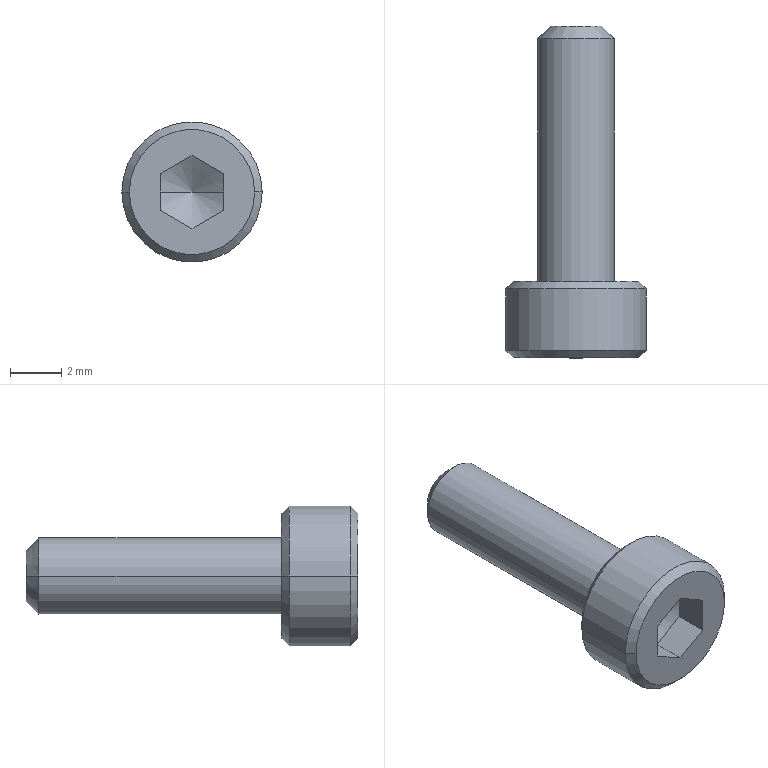Part | STEP file | BB62-M3-10L-17 | 1 solid | 27 faces | box 5.5 x 13 x 5.5 mm | volume 130.673 mm3 | plane 15 | cone 8 | cylinder 4 | commonest cylinder face diameters 3 x2 5.5 x2
STEP:
#1=CARTESIAN_POINT('',(0.,-0.8715,0.));
#2=VERTEX_POINT('',#1);
#3=CARTESIAN_POINT('',(1.435,-1.7,0.));
#4=VERTEX_POINT('',#3);
#5=CARTESIAN_POINT('',(0.,-0.8715,0.));
#6=DIRECTION('',(0.866,-0.5,0.));
#7=VECTOR('',#6,1000.);
#8=LINE('',#5,#7);
#9=EDGE_CURVE('',#2,#4,#8,.T.);
#10=ORIENTED_EDGE('',*,*,#9,.F.);
#11=CARTESIAN_POINT('',(-1.435,-1.7,0.));
#12=VERTEX_POINT('',#11);
#13=CARTESIAN_POINT('',(0.,-0.8715,0.));
#14=DIRECTION('',(-0.866,-0.5,0.));
#15=VECTOR('',#14,1000.);
#16=LINE('',#13,#15);
#17=EDGE_CURVE('',#2,#12,#16,.T.);
#18=ORIENTED_EDGE('',*,*,#17,.T.);
#19=CARTESIAN_POINT('',(-1.243,-1.7,-0.7175));
#20=VERTEX_POINT('',#19);
#21=CARTESIAN_POINT('',(0.,-1.7,0.));
#22=DIRECTION('',(0.,-1.,0.));
#23=DIRECTION('',(-1.,0.,0.));
#24=AXIS2_PLACEMENT_3D('',#21,#22,#23);
#25=CIRCLE('',#24,1.435);
#26=EDGE_CURVE('',#12,#20,#25,.T.);
#27=ORIENTED_EDGE('',*,*,#26,.T.);
#28=CARTESIAN_POINT('',(0.,-1.7,-1.435));
#29=VERTEX_POINT('',#28);
#30=CARTESIAN_POINT('',(0.,-1.7,0.));
#31=DIRECTION('',(0.,-1.,0.));
#32=DIRECTION('',(-1.,0.,0.));
#33=AXIS2_PLACEMENT_3D('',#30,#31,#32);
#34=CIRCLE('',#33,1.435);
#35=EDGE_CURVE('',#20,#29,#34,.T.);
#36=ORIENTED_EDGE('',*,*,#35,.T.);
#37=CARTESIAN_POINT('',(1.243,-1.7,-0.7175));
#38=VERTEX_POINT('',#37);
#39=CARTESIAN_POINT('',(0.,-1.7,0.));
#40=DIRECTION('',(0.,-1.,0.));
#41=DIRECTION('',(-1.,0.,0.));
#42=AXIS2_PLACEMENT_3D('',#39,#40,#41);
#43=CIRCLE('',#42,1.435);
#44=EDGE_CURVE('',#29,#38,#43,.T.);
#45=ORIENTED_EDGE('',*,*,#44,.T.);
#46=CARTESIAN_POINT('',(0.,-1.7,0.));
#47=DIRECTION('',(0.,-1.,0.));
#48=DIRECTION('',(-1.,0.,0.));
#49=AXIS2_PLACEMENT_3D('',#46,#47,#48);
#50=CIRCLE('',#49,1.435);
#51=EDGE_CURVE('',#38,#4,#50,.T.);
#52=ORIENTED_EDGE('',*,*,#51,.T.);
#53=EDGE_LOOP('',(#10,#18,#27,#36,#45,#52));
#54=FACE_OUTER_BOUND('',#53,.T.);
#55=CARTESIAN_POINT('',(0.,-1000.872,0.));
#56=DIRECTION('',(0.,-1.,0.));
#57=DIRECTION('',(1.,0.,0.));
#58=AXIS2_PLACEMENT_3D('',#55,#56,#57);
#59=CONICAL_SURFACE('',#58,1732.051,1.047);
#60=ADVANCED_FACE('',(#54),#59,.F.);
#61=CARTESIAN_POINT('',(-1.,10.,0.));
#62=VERTEX_POINT('',#61);
#63=CARTESIAN_POINT('',(1.,10.,0.));
#64=VERTEX_POINT('',#63);
#65=CARTESIAN_POINT('',(0.,10.,0.));
#66=DIRECTION('',(0.,1.,0.));
#67=DIRECTION('',(1.,0.,0.));
#68=AXIS2_PLACEMENT_3D('',#65,#66,#67);
#69=CIRCLE('',#68,1.);
#70=EDGE_CURVE('',#62,#64,#69,.T.);
#71=ORIENTED_EDGE('',*,*,#70,.F.);
#72=CARTESIAN_POINT('',(-1.5,9.5,0.));
#73=VERTEX_POINT('',#72);
#74=CARTESIAN_POINT('',(-1.,10.,0.));
#75=DIRECTION('',(-0.7071,-0.7071,0.));
#76=VECTOR('',#75,1000.);
#77=LINE('',#74,#76);
#78=EDGE_CURVE('',#62,#73,#77,.T.);
#79=ORIENTED_EDGE('',*,*,#78,.T.);
#80=CARTESIAN_POINT('',(1.5,9.5,0.));
#81=VERTEX_POINT('',#80);
#82=CARTESIAN_POINT('',(0.,9.5,0.));
#83=DIRECTION('',(0.,-1.,0.));
#84=DIRECTION('',(-1.,0.,0.));
#85=AXIS2_PLACEMENT_3D('',#82,#83,#84);
#86=CIRCLE('',#85,1.5);
#87=EDGE_CURVE('',#81,#73,#86,.T.);
#88=ORIENTED_EDGE('',*,*,#87,.F.);
#89=CARTESIAN_POINT('',(1.,10.,0.));
#90=DIRECTION('',(0.7071,-0.7071,0.));
#91=VECTOR('',#90,1000.);
#92=LINE('',#89,#91);
#93=EDGE_CURVE('',#64,#81,#92,.T.);
#94=ORIENTED_EDGE('',*,*,#93,.F.);
#95=EDGE_LOOP('',(#71,#79,#88,#94));
#96=FACE_OUTER_BOUND('',#95,.T.);
#97=CARTESIAN_POINT('',(0.,10.,0.));
#98=DIRECTION('',(0.,-1.,0.));
#99=DIRECTION('',(1.,0.,0.));
#100=AXIS2_PLACEMENT_3D('',#97,#98,#99);
#101=CONICAL_SURFACE('',#100,1.,0.7854);
#102=ADVANCED_FACE('',(#96),#101,.T.);
#103=ORIENTED_EDGE('',*,*,#87,.T.);
#104=CARTESIAN_POINT('',(-1.5,0.,0.));
#105=VERTEX_POINT('',#104);
#106=CARTESIAN_POINT('',(-1.5,9.5,0.));
#107=DIRECTION('',(0.,-1.,0.));
#108=VECTOR('',#107,1000.);
#109=LINE('',#106,#108);
#110=EDGE_CURVE('',#73,#105,#109,.T.);
#111=ORIENTED_EDGE('',*,*,#110,.T.);
#112=CARTESIAN_POINT('',(1.5,0.,0.));
#113=VERTEX_POINT('',#112);
#114=CARTESIAN_POINT('',(0.,0.,0.));
#115=DIRECTION('',(0.,-1.,0.));
#116=DIRECTION('',(-1.,0.,0.));
#117=AXIS2_PLACEMENT_3D('',#114,#115,#116);
#118=CIRCLE('',#117,1.5);
#119=EDGE_CURVE('',#113,#105,#118,.T.);
#120=ORIENTED_EDGE('',*,*,#119,.F.);
#121=CARTESIAN_POINT('',(1.5,9.5,0.));
#122=DIRECTION('',(0.,-1.,0.));
#123=VECTOR('',#122,1000.);
#124=LINE('',#121,#123);
#125=EDGE_CURVE('',#81,#113,#124,.T.);
#126=ORIENTED_EDGE('',*,*,#125,.F.);
#127=EDGE_LOOP('',(#103,#111,#120,#126));
#128=FACE_OUTER_BOUND('',#127,.T.);
#129=CARTESIAN_POINT('',(0.,9.5,0.));
#130=DIRECTION('',(0.,-1.,0.));
#131=DIRECTION('',(1.,0.,0.));
#132=AXIS2_PLACEMENT_3D('',#129,#130,#131);
#133=CYLINDRICAL_SURFACE('',#132,1.5);
#134=ADVANCED_FACE('',(#128),#133,.T.);
#135=CARTESIAN_POINT('',(2.45,-3.,0.));
#136=VERTEX_POINT('',#135);
#137=CARTESIAN_POINT('',(-2.45,-3.,0.));
#138=VERTEX_POINT('',#137);
#139=CARTESIAN_POINT('',(0.,-3.,0.));
#140=DIRECTION('',(0.,-1.,0.));
#141=DIRECTION('',(-1.,0.,0.));
#142=AXIS2_PLACEMENT_3D('',#139,#140,#141);
#143=CIRCLE('',#142,2.45);
#144=EDGE_CURVE('',#136,#138,#143,.T.);
#145=ORIENTED_EDGE('',*,*,#144,.F.);
#146=CARTESIAN_POINT('',(2.75,-2.7,0.));
#147=VERTEX_POINT('',#146);
#148=CARTESIAN_POINT('',(2.75,-2.7,0.));
#149=DIRECTION('',(0.7071,0.7071,0.));
#150=VECTOR('',#149,1000.);
#151=LINE('',#148,#150);
#152=EDGE_CURVE('',#136,#147,#151,.T.);
#153=ORIENTED_EDGE('',*,*,#152,.T.);
#154=CARTESIAN_POINT('',(-2.75,-2.7,0.));
#155=VERTEX_POINT('',#154);
#156=CARTESIAN_POINT('',(0.,-2.7,0.));
#157=DIRECTION('',(0.,-1.,0.));
#158=DIRECTION('',(-1.,0.,0.));
#159=AXIS2_PLACEMENT_3D('',#156,#157,#158);
#160=CIRCLE('',#159,2.75);
#161=EDGE_CURVE('',#147,#155,#160,.T.);
#162=ORIENTED_EDGE('',*,*,#161,.T.);
#163=CARTESIAN_POINT('',(-2.75,-2.7,0.));
#164=DIRECTION('',(-0.7071,0.7071,0.));
#165=VECTOR('',#164,1000.);
#166=LINE('',#163,#165);
#167=EDGE_CURVE('',#138,#155,#166,.T.);
#168=ORIENTED_EDGE('',*,*,#167,.F.);
#169=EDGE_LOOP('',(#145,#153,#162,#168));
#170=FACE_OUTER_BOUND('',#169,.T.);
#171=CARTESIAN_POINT('',(0.,-2.7,0.));
#172=DIRECTION('',(0.,1.,0.));
#173=DIRECTION('',(-1.,0.,0.));
#174=AXIS2_PLACEMENT_3D('',#171,#172,#173);
#175=CONICAL_SURFACE('',#174,2.75,0.7854);
#176=ADVANCED_FACE('',(#170),#175,.T.);
#177=ORIENTED_EDGE('',*,*,#161,.F.);
#178=CARTESIAN_POINT('',(2.75,-0.3,0.));
#179=VERTEX_POINT('',#178);
#180=CARTESIAN_POINT('',(2.75,-1.62,0.));
#181=DIRECTION('',(0.,1.,0.));
#182=VECTOR('',#181,1000.);
#183=LINE('',#180,#182);
#184=EDGE_CURVE('',#147,#179,#183,.T.);
#185=ORIENTED_EDGE('',*,*,#184,.T.);
#186=CARTESIAN_POINT('',(-2.75,-0.3,0.));
#187=VERTEX_POINT('',#186);
#188=CARTESIAN_POINT('',(0.,-0.3,0.));
#189=DIRECTION('',(0.,-1.,0.));
#190=DIRECTION('',(-1.,0.,0.));
#191=AXIS2_PLACEMENT_3D('',#188,#189,#190);
#192=CIRCLE('',#191,2.75);
#193=EDGE_CURVE('',#179,#187,#192,.T.);
#194=ORIENTED_EDGE('',*,*,#193,.T.);
#195=CARTESIAN_POINT('',(-2.75,-1.62,0.));
#196=DIRECTION('',(0.,1.,0.));
#197=VECTOR('',#196,1000.);
#198=LINE('',#195,#197);
#199=EDGE_CURVE('',#155,#187,#198,.T.);
#200=ORIENTED_EDGE('',*,*,#199,.F.);
#201=EDGE_LOOP('',(#177,#185,#194,#200));
#202=FACE_OUTER_BOUND('',#201,.T.);
#203=CARTESIAN_POINT('',(0.,-1.62,0.));
#204=DIRECTION('',(0.,1.,0.));
#205=DIRECTION('',(-1.,0.,0.));
#206=AXIS2_PLACEMENT_3D('',#203,#204,#205);
#207=CYLINDRICAL_SURFACE('',#206,2.75);
#208=ADVANCED_FACE('',(#202),#207,.T.);
#209=CARTESIAN_POINT('',(2.45,0.,0.));
#210=VERTEX_POINT('',#209);
#211=CARTESIAN_POINT('',(-2.45,0.,0.));
#212=VERTEX_POINT('',#211);
#213=CARTESIAN_POINT('',(0.,0.,0.));
#214=DIRECTION('',(0.,-1.,0.));
#215=DIRECTION('',(-1.,0.,0.));
#216=AXIS2_PLACEMENT_3D('',#213,#214,#215);
#217=CIRCLE('',#216,2.45);
#218=EDGE_CURVE('',#210,#212,#217,.T.);
#219=ORIENTED_EDGE('',*,*,#218,.T.);
#220=CARTESIAN_POINT('',(-2.45,0.,0.));
#221=DIRECTION('',(-0.7071,-0.7071,0.));
#222=VECTOR('',#221,1000.);
#223=LINE('',#220,#222);
#224=EDGE_CURVE('',#212,#187,#223,.T.);
#225=ORIENTED_EDGE('',*,*,#224,.T.);
#226=ORIENTED_EDGE('',*,*,#193,.F.);
#227=CARTESIAN_POINT('',(2.45,0.,0.));
#228=DIRECTION('',(0.7071,-0.7071,0.));
#229=VECTOR('',#228,1000.);
#230=LINE('',#227,#229);
#231=EDGE_CURVE('',#210,#179,#230,.T.);
#232=ORIENTED_EDGE('',*,*,#231,.F.);
#233=EDGE_LOOP('',(#219,#225,#226,#232));
#234=FACE_OUTER_BOUND('',#233,.T.);
#235=CARTESIAN_POINT('',(0.,0.,0.));
#236=DIRECTION('',(0.,-1.,0.));
#237=DIRECTION('',(1.,0.,0.));
#238=AXIS2_PLACEMENT_3D('',#235,#236,#237);
#239=CONICAL_SURFACE('',#238,2.45,0.7854);
#240=ADVANCED_FACE('',(#234),#239,.T.);
#241=CARTESIAN_POINT('',(0.,-3.,0.));
#242=DIRECTION('',(0.,-1.,0.));
#243=DIRECTION('',(-1.,0.,0.));
#244=AXIS2_PLACEMENT_3D('',#241,#242,#243);
#245=CIRCLE('',#244,2.45);
#246=EDGE_CURVE('',#138,#136,#245,.T.);
#247=ORIENTED_EDGE('',*,*,#246,.T.);
#248=ORIENTED_EDGE('',*,*,#144,.T.);
#249=EDGE_LOOP('',(#247,#248));
#250=FACE_OUTER_BOUND('',#249,.T.);
#251=CARTESIAN_POINT('',(0.,-3.,-1.435));
#252=VERTEX_POINT('',#251);
#253=CARTESIAN_POINT('',(-1.243,-3.,-0.7175));
#254=VERTEX_POINT('',#253);
#255=CARTESIAN_POINT('',(0.,-3.,-1.435));
#256=DIRECTION('',(-0.866,0.,0.5));
#257=VECTOR('',#256,1000.);
#258=LINE('',#255,#257);
#259=EDGE_CURVE('',#252,#254,#258,.T.);
#260=ORIENTED_EDGE('',*,*,#259,.T.);
#261=CARTESIAN_POINT('',(-1.243,-3.,0.7175));
#262=VERTEX_POINT('',#261);
#263=CARTESIAN_POINT('',(-1.243,-3.,-0.7175));
#264=DIRECTION('',(0.,0.,1.));
#265=VECTOR('',#264,1000.);
#266=LINE('',#263,#265);
#267=EDGE_CURVE('',#254,#262,#266,.T.);
#268=ORIENTED_EDGE('',*,*,#267,.T.);
#269=CARTESIAN_POINT('',(0.,-3.,1.435));
#270=VERTEX_POINT('',#269);
#271=CARTESIAN_POINT('',(-1.243,-3.,0.7175));
#272=DIRECTION('',(0.866,0.,0.5));
#273=VECTOR('',#272,1000.);
#274=LINE('',#271,#273);
#275=EDGE_CURVE('',#262,#270,#274,.T.);
#276=ORIENTED_EDGE('',*,*,#275,.T.);
#277=CARTESIAN_POINT('',(1.243,-3.,0.7175));
#278=VERTEX_POINT('',#277);
#279=CARTESIAN_POINT('',(0.,-3.,1.435));
#280=DIRECTION('',(0.866,0.,-0.5));
#281=VECTOR('',#280,1000.);
#282=LINE('',#279,#281);
#283=EDGE_CURVE('',#270,#278,#282,.T.);
#284=ORIENTED_EDGE('',*,*,#283,.T.);
#285=CARTESIAN_POINT('',(1.243,-3.,-0.7175));
#286=VERTEX_POINT('',#285);
#287=CARTESIAN_POINT('',(1.243,-3.,0.7175));
#288=DIRECTION('',(0.,0.,-1.));
#289=VECTOR('',#288,1000.);
#290=LINE('',#287,#289);
#291=EDGE_CURVE('',#278,#286,#290,.T.);
#292=ORIENTED_EDGE('',*,*,#291,.T.);
#293=CARTESIAN_POINT('',(1.243,-3.,-0.7175));
#294=DIRECTION('',(-0.866,0.,-0.5));
#295=VECTOR('',#294,1000.);
#296=LINE('',#293,#295);
#297=EDGE_CURVE('',#286,#252,#296,.T.);
#298=ORIENTED_EDGE('',*,*,#297,.T.);
#299=EDGE_LOOP('',(#260,#268,#276,#284,#292,#298));
#300=FACE_BOUND('',#299,.T.);
#301=CARTESIAN_POINT('',(2.45,-3.,0.));
#302=DIRECTION('',(0.,-1.,0.));
#303=DIRECTION('',(1.,0.,0.));
#304=AXIS2_PLACEMENT_3D('',#301,#302,#303);
#305=PLANE('',#304);
#306=ADVANCED_FACE('',(#250,#300),#305,.T.);
#307=ORIENTED_EDGE('',*,*,#119,.T.);
#308=CARTESIAN_POINT('',(0.,0.,0.));
#309=DIRECTION('',(0.,-1.,0.));
#310=DIRECTION('',(-1.,0.,0.));
#311=AXIS2_PLACEMENT_3D('',#308,#309,#310);
#312=CIRCLE('',#311,1.5);
#313=EDGE_CURVE('',#105,#113,#312,.T.);
#314=ORIENTED_EDGE('',*,*,#313,.T.);
#315=EDGE_LOOP('',(#307,#314));
#316=FACE_BOUND('',#315,.T.);
#317=ORIENTED_EDGE('',*,*,#218,.F.);
#318=CARTESIAN_POINT('',(0.,0.,0.));
#319=DIRECTION('',(0.,-1.,0.));
#320=DIRECTION('',(-1.,0.,0.));
#321=AXIS2_PLACEMENT_3D('',#318,#319,#320);
#322=CIRCLE('',#321,2.45);
#323=EDGE_CURVE('',#212,#210,#322,.T.);
#324=ORIENTED_EDGE('',*,*,#323,.F.);
#325=EDGE_LOOP('',(#317,#324));
#326=FACE_OUTER_BOUND('',#325,.T.);
#327=CARTESIAN_POINT('',(0.,0.,0.));
#328=DIRECTION('',(0.,1.,0.));
#329=DIRECTION('',(-1.,0.,0.));
#330=AXIS2_PLACEMENT_3D('',#327,#328,#329);
#331=PLANE('',#330);
#332=ADVANCED_FACE('',(#316,#326),#331,.T.);
#333=ORIENTED_EDGE('',*,*,#224,.F.);
#334=ORIENTED_EDGE('',*,*,#323,.T.);
#335=ORIENTED_EDGE('',*,*,#231,.T.);
#336=CARTESIAN_POINT('',(0.,-0.3,0.));
#337=DIRECTION('',(0.,-1.,0.));
#338=DIRECTION('',(-1.,0.,0.));
#339=AXIS2_PLACEMENT_3D('',#336,#337,#338);
#340=CIRCLE('',#339,2.75);
#341=EDGE_CURVE('',#187,#179,#340,.T.);
#342=ORIENTED_EDGE('',*,*,#341,.F.);
#343=EDGE_LOOP('',(#333,#334,#335,#342));
#344=FACE_OUTER_BOUND('',#343,.T.);
#345=CARTESIAN_POINT('',(0.,0.,0.));
#346=DIRECTION('',(0.,-1.,0.));
#347=DIRECTION('',(1.,0.,0.));
#348=AXIS2_PLACEMENT_3D('',#345,#346,#347);
#349=CONICAL_SURFACE('',#348,2.45,0.7854);
#350=ADVANCED_FACE('',(#344),#349,.T.);
#351=ORIENTED_EDGE('',*,*,#184,.F.);
#352=CARTESIAN_POINT('',(0.,-2.7,0.));
#353=DIRECTION('',(0.,-1.,0.));
#354=DIRECTION('',(-1.,0.,0.));
#355=AXIS2_PLACEMENT_3D('',#352,#353,#354);
#356=CIRCLE('',#355,2.75);
#357=EDGE_CURVE('',#155,#147,#356,.T.);
#358=ORIENTED_EDGE('',*,*,#357,.F.);
#359=ORIENTED_EDGE('',*,*,#199,.T.);
#360=ORIENTED_EDGE('',*,*,#341,.T.);
#361=EDGE_LOOP('',(#351,#358,#359,#360));
#362=FACE_OUTER_BOUND('',#361,.T.);
#363=CARTESIAN_POINT('',(0.,-1.62,0.));
#364=DIRECTION('',(0.,1.,0.));
#365=DIRECTION('',(-1.,0.,0.));
#366=AXIS2_PLACEMENT_3D('',#363,#364,#365);
#367=CYLINDRICAL_SURFACE('',#366,2.75);
#368=ADVANCED_FACE('',(#362),#367,.T.);
#369=ORIENTED_EDGE('',*,*,#152,.F.);
#370=ORIENTED_EDGE('',*,*,#246,.F.);
#371=ORIENTED_EDGE('',*,*,#167,.T.);
#372=ORIENTED_EDGE('',*,*,#357,.T.);
#373=EDGE_LOOP('',(#369,#370,#371,#372));
#374=FACE_OUTER_BOUND('',#373,.T.);
#375=CARTESIAN_POINT('',(0.,-2.7,0.));
#376=DIRECTION('',(0.,1.,0.));
#377=DIRECTION('',(-1.,0.,0.));
#378=AXIS2_PLACEMENT_3D('',#375,#376,#377);
#379=CONICAL_SURFACE('',#378,2.75,0.7854);
#380=ADVANCED_FACE('',(#374),#379,.T.);
#381=ORIENTED_EDGE('',*,*,#110,.F.);
#382=CARTESIAN_POINT('',(0.,9.5,0.));
#383=DIRECTION('',(0.,-1.,0.));
#384=DIRECTION('',(-1.,0.,0.));
#385=AXIS2_PLACEMENT_3D('',#382,#383,#384);
#386=CIRCLE('',#385,1.5);
#387=EDGE_CURVE('',#73,#81,#386,.T.);
#388=ORIENTED_EDGE('',*,*,#387,.T.);
#389=ORIENTED_EDGE('',*,*,#125,.T.);
#390=ORIENTED_EDGE('',*,*,#313,.F.);
#391=EDGE_LOOP('',(#381,#388,#389,#390));
#392=FACE_OUTER_BOUND('',#391,.T.);
#393=CARTESIAN_POINT('',(0.,9.5,0.));
#394=DIRECTION('',(0.,-1.,0.));
#395=DIRECTION('',(1.,0.,0.));
#396=AXIS2_PLACEMENT_3D('',#393,#394,#395);
#397=CYLINDRICAL_SURFACE('',#396,1.5);
#398=ADVANCED_FACE('',(#392),#397,.T.);
#399=CARTESIAN_POINT('',(0.,10.,0.));
#400=DIRECTION('',(0.,1.,0.));
#401=DIRECTION('',(1.,0.,0.));
#402=AXIS2_PLACEMENT_3D('',#399,#400,#401);
#403=CIRCLE('',#402,1.);
#404=EDGE_CURVE('',#64,#62,#403,.T.);
#405=ORIENTED_EDGE('',*,*,#404,.T.);
#406=ORIENTED_EDGE('',*,*,#70,.T.);
#407=EDGE_LOOP('',(#405,#406));
#408=FACE_OUTER_BOUND('',#407,.T.);
#409=CARTESIAN_POINT('',(0.,10.,0.));
#410=DIRECTION('',(0.,1.,0.));
#411=DIRECTION('',(-1.,0.,0.));
#412=AXIS2_PLACEMENT_3D('',#409,#410,#411);
#413=PLANE('',#412);
#414=ADVANCED_FACE('',(#408),#413,.T.);
#415=ORIENTED_EDGE('',*,*,#78,.F.);
#416=ORIENTED_EDGE('',*,*,#404,.F.);
#417=ORIENTED_EDGE('',*,*,#93,.T.);
#418=ORIENTED_EDGE('',*,*,#387,.F.);
#419=EDGE_LOOP('',(#415,#416,#417,#418));
#420=FACE_OUTER_BOUND('',#419,.T.);
#421=CARTESIAN_POINT('',(0.,10.,0.));
#422=DIRECTION('',(0.,-1.,0.));
#423=DIRECTION('',(1.,0.,0.));
#424=AXIS2_PLACEMENT_3D('',#421,#422,#423);
#425=CONICAL_SURFACE('',#424,1.,0.7854);
#426=ADVANCED_FACE('',(#420),#425,.T.);
#427=CARTESIAN_POINT('',(1.243,-1.7,-0.7175));
#428=DIRECTION('',(-0.866,0.,-0.5));
#429=VECTOR('',#428,1000.);
#430=LINE('',#427,#429);
#431=EDGE_CURVE('',#38,#29,#430,.T.);
#432=ORIENTED_EDGE('',*,*,#431,.T.);
#433=CARTESIAN_POINT('',(0.,-3.,-1.435));
#434=DIRECTION('',(0.,1.,0.));
#435=VECTOR('',#434,1000.);
#436=LINE('',#433,#435);
#437=EDGE_CURVE('',#252,#29,#436,.T.);
#438=ORIENTED_EDGE('',*,*,#437,.F.);
#439=ORIENTED_EDGE('',*,*,#297,.F.);
#440=CARTESIAN_POINT('',(1.243,-3.,-0.7175));
#441=DIRECTION('',(0.,1.,0.));
#442=VECTOR('',#441,1000.);
#443=LINE('',#440,#442);
#444=EDGE_CURVE('',#286,#38,#443,.T.);
#445=ORIENTED_EDGE('',*,*,#444,.T.);
#446=EDGE_LOOP('',(#432,#438,#439,#445));
#447=FACE_OUTER_BOUND('',#446,.T.);
#448=CARTESIAN_POINT('',(1.243,-3.,-0.7175));
#449=DIRECTION('',(-0.5,0.,0.866));
#450=DIRECTION('',(0.866,0.,0.5));
#451=AXIS2_PLACEMENT_3D('',#448,#449,#450);
#452=PLANE('',#451);
#453=ADVANCED_FACE('',(#447),#452,.T.);
#454=CARTESIAN_POINT('',(0.,-1.7,-1.435));
#455=DIRECTION('',(-0.866,0.,0.5));
#456=VECTOR('',#455,1000.);
#457=LINE('',#454,#456);
#458=EDGE_CURVE('',#29,#20,#457,.T.);
#459=ORIENTED_EDGE('',*,*,#458,.T.);
#460=CARTESIAN_POINT('',(-1.243,-3.,-0.7175));
#461=DIRECTION('',(0.,1.,0.));
#462=VECTOR('',#461,1000.);
#463=LINE('',#460,#462);
#464=EDGE_CURVE('',#254,#20,#463,.T.);
#465=ORIENTED_EDGE('',*,*,#464,.F.);
#466=ORIENTED_EDGE('',*,*,#259,.F.);
#467=ORIENTED_EDGE('',*,*,#437,.T.);
#468=EDGE_LOOP('',(#459,#465,#466,#467));
#469=FACE_OUTER_BOUND('',#468,.T.);
#470=CARTESIAN_POINT('',(0.,-3.,-1.435));
#471=DIRECTION('',(0.5,0.,0.866));
#472=DIRECTION('',(0.866,0.,-0.5));
#473=AXIS2_PLACEMENT_3D('',#470,#471,#472);
#474=PLANE('',#473);
#475=ADVANCED_FACE('',(#469),#474,.T.);
#476=CARTESIAN_POINT('',(-1.243,-1.7,0.7175));
#477=VERTEX_POINT('',#476);
#478=CARTESIAN_POINT('',(-1.243,-1.7,-0.7175));
#479=DIRECTION('',(0.,0.,1.));
#480=VECTOR('',#479,1000.);
#481=LINE('',#478,#480);
#482=EDGE_CURVE('',#20,#477,#481,.T.);
#483=ORIENTED_EDGE('',*,*,#482,.T.);
#484=CARTESIAN_POINT('',(-1.243,-3.,0.7175));
#485=DIRECTION('',(0.,1.,0.));
#486=VECTOR('',#485,1000.);
#487=LINE('',#484,#486);
#488=EDGE_CURVE('',#262,#477,#487,.T.);
#489=ORIENTED_EDGE('',*,*,#488,.F.);
#490=ORIENTED_EDGE('',*,*,#267,.F.);
#491=ORIENTED_EDGE('',*,*,#464,.T.);
#492=EDGE_LOOP('',(#483,#489,#490,#491));
#493=FACE_OUTER_BOUND('',#492,.T.);
#494=CARTESIAN_POINT('',(-1.243,-3.,-0.7175));
#495=DIRECTION('',(1.,0.,0.));
#496=DIRECTION('',(0.,0.,-1.));
#497=AXIS2_PLACEMENT_3D('',#494,#495,#496);
#498=PLANE('',#497);
#499=ADVANCED_FACE('',(#493),#498,.T.);
#500=CARTESIAN_POINT('',(0.,-1.7,1.435));
#501=VERTEX_POINT('',#500);
#502=CARTESIAN_POINT('',(-1.243,-1.7,0.7175));
#503=DIRECTION('',(0.866,0.,0.5));
#504=VECTOR('',#503,1000.);
#505=LINE('',#502,#504);
#506=EDGE_CURVE('',#477,#501,#505,.T.);
#507=ORIENTED_EDGE('',*,*,#506,.T.);
#508=CARTESIAN_POINT('',(0.,-3.,1.435));
#509=DIRECTION('',(0.,1.,0.));
#510=VECTOR('',#509,1000.);
#511=LINE('',#508,#510);
#512=EDGE_CURVE('',#270,#501,#511,.T.);
#513=ORIENTED_EDGE('',*,*,#512,.F.);
#514=ORIENTED_EDGE('',*,*,#275,.F.);
#515=ORIENTED_EDGE('',*,*,#488,.T.);
#516=EDGE_LOOP('',(#507,#513,#514,#515));
#517=FACE_OUTER_BOUND('',#516,.T.);
#518=CARTESIAN_POINT('',(-1.243,-3.,0.7175));
#519=DIRECTION('',(0.5,0.,-0.866));
#520=DIRECTION('',(-0.866,0.,-0.5));
#521=AXIS2_PLACEMENT_3D('',#518,#519,#520);
#522=PLANE('',#521);
#523=ADVANCED_FACE('',(#517),#522,.T.);
#524=CARTESIAN_POINT('',(1.243,-1.7,0.7175));
#525=VERTEX_POINT('',#524);
#526=CARTESIAN_POINT('',(0.,-1.7,1.435));
#527=DIRECTION('',(0.866,0.,-0.5));
#528=VECTOR('',#527,1000.);
#529=LINE('',#526,#528);
#530=EDGE_CURVE('',#501,#525,#529,.T.);
#531=ORIENTED_EDGE('',*,*,#530,.T.);
#532=CARTESIAN_POINT('',(1.243,-3.,0.7175));
#533=DIRECTION('',(0.,1.,0.));
#534=VECTOR('',#533,1000.);
#535=LINE('',#532,#534);
#536=EDGE_CURVE('',#278,#525,#535,.T.);
#537=ORIENTED_EDGE('',*,*,#536,.F.);
#538=ORIENTED_EDGE('',*,*,#283,.F.);
#539=ORIENTED_EDGE('',*,*,#512,.T.);
#540=EDGE_LOOP('',(#531,#537,#538,#539));
#541=FACE_OUTER_BOUND('',#540,.T.);
#542=CARTESIAN_POINT('',(0.,-3.,1.435));
#543=DIRECTION('',(-0.5,0.,-0.866));
#544=DIRECTION('',(-0.866,0.,0.5));
#545=AXIS2_PLACEMENT_3D('',#542,#543,#544);
#546=PLANE('',#545);
#547=ADVANCED_FACE('',(#541),#546,.T.);
#548=CARTESIAN_POINT('',(1.243,-1.7,0.7175));
#549=DIRECTION('',(0.,0.,-1.));
#550=VECTOR('',#549,1000.);
#551=LINE('',#548,#550);
#552=EDGE_CURVE('',#525,#38,#551,.T.);
#553=ORIENTED_EDGE('',*,*,#552,.T.);
#554=ORIENTED_EDGE('',*,*,#444,.F.);
#555=ORIENTED_EDGE('',*,*,#291,.F.);
#556=ORIENTED_EDGE('',*,*,#536,.T.);
#557=EDGE_LOOP('',(#553,#554,#555,#556));
#558=FACE_OUTER_BOUND('',#557,.T.);
#559=CARTESIAN_POINT('',(1.243,-3.,0.7175));
#560=DIRECTION('',(-1.,0.,0.));
#561=DIRECTION('',(0.,0.,1.));
#562=AXIS2_PLACEMENT_3D('',#559,#560,#561);
#563=PLANE('',#562);
#564=ADVANCED_FACE('',(#558),#563,.T.);
#565=ORIENTED_EDGE('',*,*,#431,.F.);
#566=ORIENTED_EDGE('',*,*,#44,.F.);
#567=EDGE_LOOP('',(#565,#566));
#568=FACE_OUTER_BOUND('',#567,.T.);
#569=CARTESIAN_POINT('',(0.,-1.7,0.));
#570=DIRECTION('',(0.,-1.,0.));
#571=DIRECTION('',(1.,0.,0.));
#572=AXIS2_PLACEMENT_3D('',#569,#570,#571);
#573=PLANE('',#572);
#574=ADVANCED_FACE('',(#568),#573,.F.);
#575=ORIENTED_EDGE('',*,*,#552,.F.);
#576=CARTESIAN_POINT('',(0.,-1.7,0.));
#577=DIRECTION('',(0.,-1.,0.));
#578=DIRECTION('',(-1.,0.,0.));
#579=AXIS2_PLACEMENT_3D('',#576,#577,#578);
#580=CIRCLE('',#579,1.435);
#581=EDGE_CURVE('',#4,#525,#580,.T.);
#582=ORIENTED_EDGE('',*,*,#581,.F.);
#583=ORIENTED_EDGE('',*,*,#51,.F.);
#584=EDGE_LOOP('',(#575,#582,#583));
#585=FACE_OUTER_BOUND('',#584,.T.);
#586=CARTESIAN_POINT('',(0.,-1.7,0.));
#587=DIRECTION('',(0.,-1.,0.));
#588=DIRECTION('',(1.,0.,0.));
#589=AXIS2_PLACEMENT_3D('',#586,#587,#588);
#590=PLANE('',#589);
#591=ADVANCED_FACE('',(#585),#590,.F.);
#592=ORIENTED_EDGE('',*,*,#530,.F.);
#593=CARTESIAN_POINT('',(0.,-1.7,0.));
#594=DIRECTION('',(0.,-1.,0.));
#595=DIRECTION('',(-1.,0.,0.));
#596=AXIS2_PLACEMENT_3D('',#593,#594,#595);
#597=CIRCLE('',#596,1.435);
#598=EDGE_CURVE('',#525,#501,#597,.T.);
#599=ORIENTED_EDGE('',*,*,#598,.F.);
#600=EDGE_LOOP('',(#592,#599));
#601=FACE_OUTER_BOUND('',#600,.T.);
#602=CARTESIAN_POINT('',(0.,-1.7,0.));
#603=DIRECTION('',(0.,-1.,0.));
#604=DIRECTION('',(1.,0.,0.));
#605=AXIS2_PLACEMENT_3D('',#602,#603,#604);
#606=PLANE('',#605);
#607=ADVANCED_FACE('',(#601),#606,.F.);
#608=ORIENTED_EDGE('',*,*,#506,.F.);
#609=CARTESIAN_POINT('',(0.,-1.7,0.));
#610=DIRECTION('',(0.,-1.,0.));
#611=DIRECTION('',(-1.,0.,0.));
#612=AXIS2_PLACEMENT_3D('',#609,#610,#611);
#613=CIRCLE('',#612,1.435);
#614=EDGE_CURVE('',#501,#477,#613,.T.);
#615=ORIENTED_EDGE('',*,*,#614,.F.);
#616=EDGE_LOOP('',(#608,#615));
#617=FACE_OUTER_BOUND('',#616,.T.);
#618=CARTESIAN_POINT('',(0.,-1.7,0.));
#619=DIRECTION('',(0.,-1.,0.));
#620=DIRECTION('',(1.,0.,0.));
#621=AXIS2_PLACEMENT_3D('',#618,#619,#620);
#622=PLANE('',#621);
#623=ADVANCED_FACE('',(#617),#622,.F.);
#624=ORIENTED_EDGE('',*,*,#482,.F.);
#625=ORIENTED_EDGE('',*,*,#26,.F.);
#626=CARTESIAN_POINT('',(0.,-1.7,0.));
#627=DIRECTION('',(0.,-1.,0.));
#628=DIRECTION('',(-1.,0.,0.));
#629=AXIS2_PLACEMENT_3D('',#626,#627,#628);
#630=CIRCLE('',#629,1.435);
#631=EDGE_CURVE('',#477,#12,#630,.T.);
#632=ORIENTED_EDGE('',*,*,#631,.F.);
#633=EDGE_LOOP('',(#624,#625,#632));
#634=FACE_OUTER_BOUND('',#633,.T.);
#635=CARTESIAN_POINT('',(0.,-1.7,0.));
#636=DIRECTION('',(0.,-1.,0.));
#637=DIRECTION('',(1.,0.,0.));
#638=AXIS2_PLACEMENT_3D('',#635,#636,#637);
#639=PLANE('',#638);
#640=ADVANCED_FACE('',(#634),#639,.F.);
#641=ORIENTED_EDGE('',*,*,#458,.F.);
#642=ORIENTED_EDGE('',*,*,#35,.F.);
#643=EDGE_LOOP('',(#641,#642));
#644=FACE_OUTER_BOUND('',#643,.T.);
#645=CARTESIAN_POINT('',(0.,-1.7,0.));
#646=DIRECTION('',(0.,-1.,0.));
#647=DIRECTION('',(1.,0.,0.));
#648=AXIS2_PLACEMENT_3D('',#645,#646,#647);
#649=PLANE('',#648);
#650=ADVANCED_FACE('',(#644),#649,.F.);
#651=ORIENTED_EDGE('',*,*,#17,.F.);
#652=ORIENTED_EDGE('',*,*,#9,.T.);
#653=ORIENTED_EDGE('',*,*,#581,.T.);
#654=ORIENTED_EDGE('',*,*,#598,.T.);
#655=ORIENTED_EDGE('',*,*,#614,.T.);
#656=ORIENTED_EDGE('',*,*,#631,.T.);
#657=EDGE_LOOP('',(#651,#652,#653,#654,#655,#656));
#658=FACE_OUTER_BOUND('',#657,.T.);
#659=CARTESIAN_POINT('',(0.,-1000.872,0.));
#660=DIRECTION('',(0.,-1.,0.));
#661=DIRECTION('',(1.,0.,0.));
#662=AXIS2_PLACEMENT_3D('',#659,#660,#661);
#663=CONICAL_SURFACE('',#662,1732.051,1.047);
#664=ADVANCED_FACE('',(#658),#663,.F.);
#665=CLOSED_SHELL('',(#60,#102,#134,#176,#208,#240,#306,#332,#350,#368,#380,#398,#414,#426,#453,#475,#499,#523,#547,#564,#574,#591,#607,#623,#640,#650,#664));
#666=MANIFOLD_SOLID_BREP('',#665);
#667=CARTESIAN_POINT('',(0.,0.,0.));
#668=DIRECTION('',(0.,0.,1.));
#669=DIRECTION('',(1.,0.,0.));
#670=AXIS2_PLACEMENT_3D('',#667,#668,#669);
#671=(LENGTH_UNIT()NAMED_UNIT(*)SI_UNIT(.MILLI.,.METRE.));
#672=UNCERTAINTY_MEASURE_WITH_UNIT(LENGTH_MEASURE(0.00001),#671,'','');
#673=(NAMED_UNIT(*)PLANE_ANGLE_UNIT()SI_UNIT($,.RADIAN.));
#674=(NAMED_UNIT(*)SI_UNIT($,.STERADIAN.)SOLID_ANGLE_UNIT());
#675=(GEOMETRIC_REPRESENTATION_CONTEXT(3)GLOBAL_UNCERTAINTY_ASSIGNED_CONTEXT((#672))GLOBAL_UNIT_ASSIGNED_CONTEXT((#671,#673,#674))REPRESENTATION_CONTEXT('',''));
#676=ADVANCED_BREP_SHAPE_REPRESENTATION('',(#666,#670),#675);